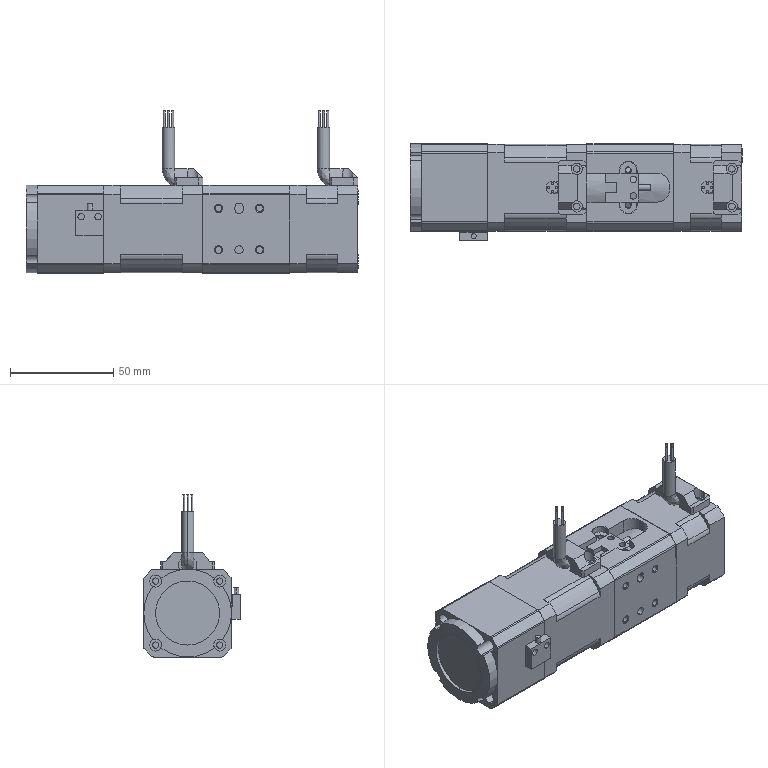Part | SolidWorks | features BaseBody 1 | 1 solid | 593 faces | box 160.8 x 46.8 x 78.5 mm | volume 260990 mm3 | cylinder 274 | plane 245 | cone 66 | spline 8 | commonest cylinder face diameters 3.3 x32 2 x28 3.2 x28 2.5 x26 8 x18 1 x16